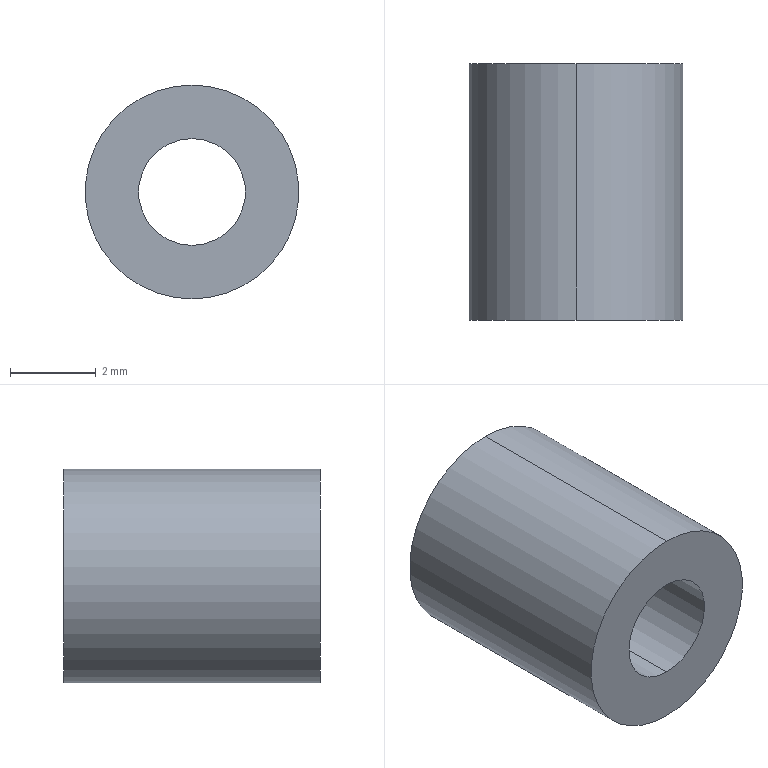Part | SolidWorks | features Extrusion 1, HoleWzd 1 | 1 solid | 6 faces | box 5 x 6 x 5 mm | volume 88.357 mm3 | cylinder 4 | plane 2 | commonest cylinder face diameters 2.5 x2 5 x2
STEP:
#1=CARTESIAN_POINT('',(0.,0.,-1.25));
#2=VERTEX_POINT('',#1);
#3=CARTESIAN_POINT('',(0.,0.,1.25));
#4=VERTEX_POINT('',#3);
#5=CARTESIAN_POINT('',(0.,0.,0.));
#6=DIRECTION('',(0.,1.,0.));
#7=DIRECTION('',(0.,0.,1.));
#8=AXIS2_PLACEMENT_3D('',#5,#6,#7);
#9=CIRCLE('',#8,1.25);
#10=EDGE_CURVE('',#2,#4,#9,.T.);
#11=ORIENTED_EDGE('',*,*,#10,.F.);
#12=CARTESIAN_POINT('',(0.,6.,-1.25));
#13=VERTEX_POINT('',#12);
#14=CARTESIAN_POINT('',(0.,6.,-1.25));
#15=DIRECTION('',(0.,1.,0.));
#16=VECTOR('',#15,1000.);
#17=LINE('',#14,#16);
#18=EDGE_CURVE('',#2,#13,#17,.T.);
#19=ORIENTED_EDGE('',*,*,#18,.T.);
#20=CARTESIAN_POINT('',(0.,6.,1.25));
#21=VERTEX_POINT('',#20);
#22=CARTESIAN_POINT('',(0.,6.,0.));
#23=DIRECTION('',(0.,1.,0.));
#24=DIRECTION('',(0.,0.,1.));
#25=AXIS2_PLACEMENT_3D('',#22,#23,#24);
#26=CIRCLE('',#25,1.25);
#27=EDGE_CURVE('',#13,#21,#26,.T.);
#28=ORIENTED_EDGE('',*,*,#27,.T.);
#29=CARTESIAN_POINT('',(0.,6.,1.25));
#30=DIRECTION('',(0.,1.,0.));
#31=VECTOR('',#30,1000.);
#32=LINE('',#29,#31);
#33=EDGE_CURVE('',#4,#21,#32,.T.);
#34=ORIENTED_EDGE('',*,*,#33,.F.);
#35=EDGE_LOOP('',(#11,#19,#28,#34));
#36=FACE_OUTER_BOUND('',#35,.T.);
#37=CARTESIAN_POINT('',(0.,6.,0.));
#38=DIRECTION('',(0.,1.,0.));
#39=DIRECTION('',(0.,0.,1.));
#40=AXIS2_PLACEMENT_3D('',#37,#38,#39);
#41=CYLINDRICAL_SURFACE('',#40,1.25);
#42=ADVANCED_FACE('',(#36),#41,.F.);
#43=CARTESIAN_POINT('',(0.,6.,2.5));
#44=VERTEX_POINT('',#43);
#45=CARTESIAN_POINT('',(0.,6.,-2.5));
#46=VERTEX_POINT('',#45);
#47=CARTESIAN_POINT('',(0.,6.,0.));
#48=DIRECTION('',(0.,1.,0.));
#49=DIRECTION('',(0.,0.,1.));
#50=AXIS2_PLACEMENT_3D('',#47,#48,#49);
#51=CIRCLE('',#50,2.5);
#52=EDGE_CURVE('',#44,#46,#51,.T.);
#53=ORIENTED_EDGE('',*,*,#52,.F.);
#54=CARTESIAN_POINT('',(0.,0.,2.5));
#55=VERTEX_POINT('',#54);
#56=CARTESIAN_POINT('',(0.,6.,2.5));
#57=DIRECTION('',(0.,-1.,0.));
#58=VECTOR('',#57,1000.);
#59=LINE('',#56,#58);
#60=EDGE_CURVE('',#44,#55,#59,.T.);
#61=ORIENTED_EDGE('',*,*,#60,.T.);
#62=CARTESIAN_POINT('',(0.,0.,-2.5));
#63=VERTEX_POINT('',#62);
#64=CARTESIAN_POINT('',(0.,0.,0.));
#65=DIRECTION('',(0.,1.,0.));
#66=DIRECTION('',(0.,0.,1.));
#67=AXIS2_PLACEMENT_3D('',#64,#65,#66);
#68=CIRCLE('',#67,2.5);
#69=EDGE_CURVE('',#55,#63,#68,.T.);
#70=ORIENTED_EDGE('',*,*,#69,.T.);
#71=CARTESIAN_POINT('',(0.,6.,-2.5));
#72=DIRECTION('',(0.,-1.,0.));
#73=VECTOR('',#72,1000.);
#74=LINE('',#71,#73);
#75=EDGE_CURVE('',#46,#63,#74,.T.);
#76=ORIENTED_EDGE('',*,*,#75,.F.);
#77=EDGE_LOOP('',(#53,#61,#70,#76));
#78=FACE_OUTER_BOUND('',#77,.T.);
#79=CARTESIAN_POINT('',(0.,6.,0.));
#80=DIRECTION('',(0.,-1.,0.));
#81=DIRECTION('',(0.,0.,-1.));
#82=AXIS2_PLACEMENT_3D('',#79,#80,#81);
#83=CYLINDRICAL_SURFACE('',#82,2.5);
#84=ADVANCED_FACE('',(#78),#83,.T.);
#85=ORIENTED_EDGE('',*,*,#60,.F.);
#86=CARTESIAN_POINT('',(0.,6.,0.));
#87=DIRECTION('',(0.,1.,0.));
#88=DIRECTION('',(0.,0.,1.));
#89=AXIS2_PLACEMENT_3D('',#86,#87,#88);
#90=CIRCLE('',#89,2.5);
#91=EDGE_CURVE('',#46,#44,#90,.T.);
#92=ORIENTED_EDGE('',*,*,#91,.F.);
#93=ORIENTED_EDGE('',*,*,#75,.T.);
#94=CARTESIAN_POINT('',(0.,0.,0.));
#95=DIRECTION('',(0.,1.,0.));
#96=DIRECTION('',(0.,0.,1.));
#97=AXIS2_PLACEMENT_3D('',#94,#95,#96);
#98=CIRCLE('',#97,2.5);
#99=EDGE_CURVE('',#63,#55,#98,.T.);
#100=ORIENTED_EDGE('',*,*,#99,.T.);
#101=EDGE_LOOP('',(#85,#92,#93,#100));
#102=FACE_OUTER_BOUND('',#101,.T.);
#103=CARTESIAN_POINT('',(0.,6.,0.));
#104=DIRECTION('',(0.,-1.,0.));
#105=DIRECTION('',(0.,0.,-1.));
#106=AXIS2_PLACEMENT_3D('',#103,#104,#105);
#107=CYLINDRICAL_SURFACE('',#106,2.5);
#108=ADVANCED_FACE('',(#102),#107,.T.);
#109=CARTESIAN_POINT('',(0.,6.,0.));
#110=DIRECTION('',(0.,1.,0.));
#111=DIRECTION('',(0.,0.,1.));
#112=AXIS2_PLACEMENT_3D('',#109,#110,#111);
#113=CIRCLE('',#112,1.25);
#114=EDGE_CURVE('',#21,#13,#113,.T.);
#115=ORIENTED_EDGE('',*,*,#114,.F.);
#116=ORIENTED_EDGE('',*,*,#27,.F.);
#117=EDGE_LOOP('',(#115,#116));
#118=FACE_BOUND('',#117,.T.);
#119=ORIENTED_EDGE('',*,*,#91,.T.);
#120=ORIENTED_EDGE('',*,*,#52,.T.);
#121=EDGE_LOOP('',(#119,#120));
#122=FACE_OUTER_BOUND('',#121,.T.);
#123=CARTESIAN_POINT('',(0.,6.,0.));
#124=DIRECTION('',(0.,1.,0.));
#125=DIRECTION('',(0.,0.,1.));
#126=AXIS2_PLACEMENT_3D('',#123,#124,#125);
#127=PLANE('',#126);
#128=ADVANCED_FACE('',(#118,#122),#127,.T.);
#129=CARTESIAN_POINT('',(0.,0.,0.));
#130=DIRECTION('',(0.,1.,0.));
#131=DIRECTION('',(0.,0.,1.));
#132=AXIS2_PLACEMENT_3D('',#129,#130,#131);
#133=CIRCLE('',#132,1.25);
#134=EDGE_CURVE('',#4,#2,#133,.T.);
#135=ORIENTED_EDGE('',*,*,#134,.T.);
#136=ORIENTED_EDGE('',*,*,#10,.T.);
#137=EDGE_LOOP('',(#135,#136));
#138=FACE_BOUND('',#137,.T.);
#139=ORIENTED_EDGE('',*,*,#99,.F.);
#140=ORIENTED_EDGE('',*,*,#69,.F.);
#141=EDGE_LOOP('',(#139,#140));
#142=FACE_OUTER_BOUND('',#141,.T.);
#143=CARTESIAN_POINT('',(0.,0.,0.));
#144=DIRECTION('',(0.,1.,0.));
#145=DIRECTION('',(0.,0.,1.));
#146=AXIS2_PLACEMENT_3D('',#143,#144,#145);
#147=PLANE('',#146);
#148=ADVANCED_FACE('',(#138,#142),#147,.F.);
#149=ORIENTED_EDGE('',*,*,#18,.F.);
#150=ORIENTED_EDGE('',*,*,#134,.F.);
#151=ORIENTED_EDGE('',*,*,#33,.T.);
#152=ORIENTED_EDGE('',*,*,#114,.T.);
#153=EDGE_LOOP('',(#149,#150,#151,#152));
#154=FACE_OUTER_BOUND('',#153,.T.);
#155=CARTESIAN_POINT('',(0.,6.,0.));
#156=DIRECTION('',(0.,1.,0.));
#157=DIRECTION('',(0.,0.,1.));
#158=AXIS2_PLACEMENT_3D('',#155,#156,#157);
#159=CYLINDRICAL_SURFACE('',#158,1.25);
#160=ADVANCED_FACE('',(#154),#159,.F.);
#161=CLOSED_SHELL('',(#42,#84,#108,#128,#148,#160));
#162=MANIFOLD_SOLID_BREP('',#161);
#163=CARTESIAN_POINT('',(0.,0.,0.));
#164=DIRECTION('',(0.,0.,1.));
#165=DIRECTION('',(1.,0.,0.));
#166=AXIS2_PLACEMENT_3D('',#163,#164,#165);
#167=(LENGTH_UNIT()NAMED_UNIT(*)SI_UNIT(.MILLI.,.METRE.));
#168=UNCERTAINTY_MEASURE_WITH_UNIT(LENGTH_MEASURE(0.00001),#167,'','');
#169=(NAMED_UNIT(*)PLANE_ANGLE_UNIT()SI_UNIT($,.RADIAN.));
#170=(NAMED_UNIT(*)SI_UNIT($,.STERADIAN.)SOLID_ANGLE_UNIT());
#171=(GEOMETRIC_REPRESENTATION_CONTEXT(3)GLOBAL_UNCERTAINTY_ASSIGNED_CONTEXT((#168))GLOBAL_UNIT_ASSIGNED_CONTEXT((#167,#169,#170))REPRESENTATION_CONTEXT('',''));
#172=ADVANCED_BREP_SHAPE_REPRESENTATION('',(#162,#166),#171);